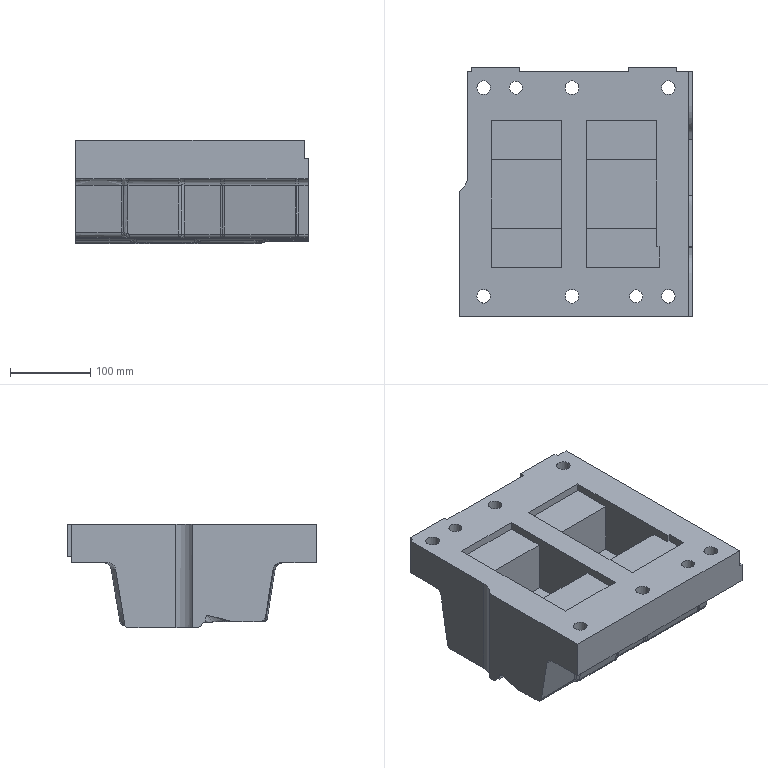Part | NX | features solid 2 | 1 solid | 246 faces | box 290 x 310 x 129.453 mm | volume 6859880 mm3 | spline 108 | plane 79 | cylinder 58 | sphere 1 | commonest cylinder face diameters 12 x16 10 x7 20 x7 8 x6 17 x6 26 x6